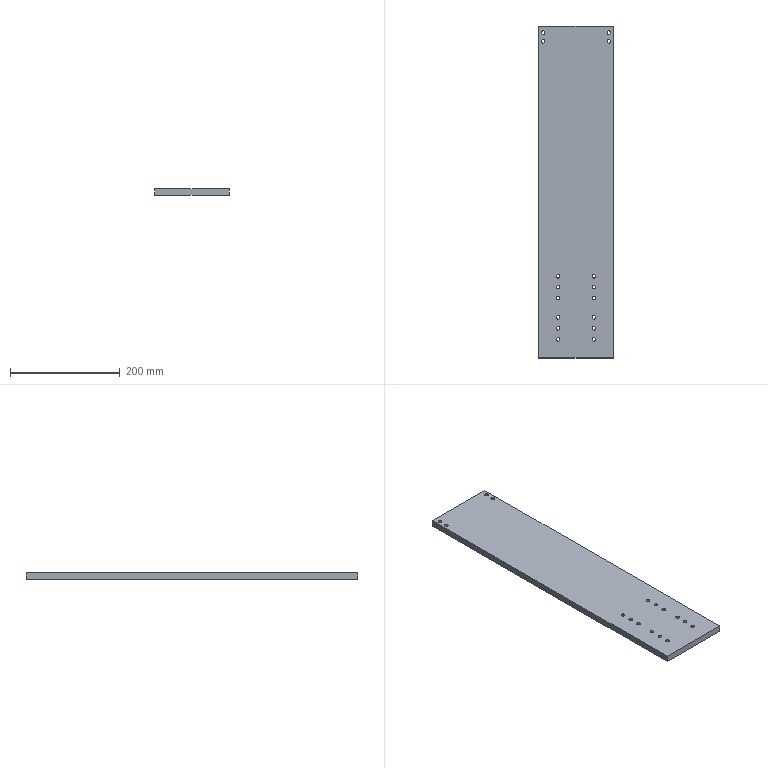Part | SolidWorks | features HoleWzd 3, Extrusion 1 | 1 solid | 102 faces | box 135 x 605 x 12 mm | volume 965539 mm3 | cylinder 72 | plane 22 | cone 8 | commonest cylinder face diameters 6.6 x32 11 x32 5 x8